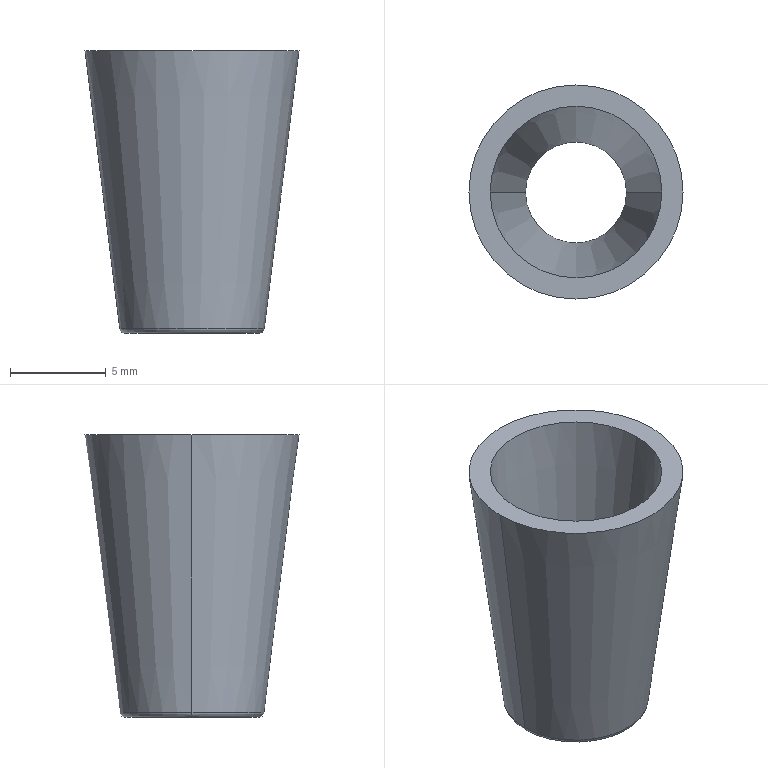Part | SolidWorks | features BaseBody 1 | 1 solid | 8 faces | box 11.2 x 11.2 x 14.8 mm | volume 424.456 mm3 | cone 4 | plane 2 | torus 2
STEP:
#1=CARTESIAN_POINT('',(-298.418,-272.746,351.634));
#2=VERTEX_POINT('',#1);
#3=CARTESIAN_POINT('',(-293.135,-272.746,351.634));
#4=VERTEX_POINT('',#3);
#5=CARTESIAN_POINT('',(-295.776,-272.746,351.634));
#6=DIRECTION('',(0.,0.,-1.));
#7=DIRECTION('',(-1.,0.,0.));
#8=AXIS2_PLACEMENT_3D('',#5,#6,#7);
#9=CIRCLE('',#8,2.641);
#10=EDGE_CURVE('',#2,#4,#9,.T.);
#11=ORIENTED_EDGE('',*,*,#10,.F.);
#12=CARTESIAN_POINT('',(-295.776,-272.746,351.634));
#13=DIRECTION('',(0.,0.,-1.));
#14=DIRECTION('',(1.,0.,0.));
#15=AXIS2_PLACEMENT_3D('',#12,#13,#14);
#16=CIRCLE('',#15,2.641);
#17=EDGE_CURVE('',#4,#2,#16,.T.);
#18=ORIENTED_EDGE('',*,*,#17,.F.);
#19=EDGE_LOOP('',(#11,#18));
#20=FACE_BOUND('',#19,.T.);
#21=CARTESIAN_POINT('',(-299.262,-272.746,351.634));
#22=VERTEX_POINT('',#21);
#23=CARTESIAN_POINT('',(-292.291,-272.746,351.634));
#24=VERTEX_POINT('',#23);
#25=CARTESIAN_POINT('',(-295.776,-272.746,351.634));
#26=DIRECTION('',(0.,0.,1.));
#27=DIRECTION('',(0.9995,-0.03162,0.));
#28=AXIS2_PLACEMENT_3D('',#25,#26,#27);
#29=CIRCLE('',#28,3.485);
#30=EDGE_CURVE('',#22,#24,#29,.T.);
#31=ORIENTED_EDGE('',*,*,#30,.F.);
#32=CARTESIAN_POINT('',(-295.776,-272.746,351.634));
#33=DIRECTION('',(0.,0.,1.));
#34=DIRECTION('',(-0.9995,0.03162,0.));
#35=AXIS2_PLACEMENT_3D('',#32,#33,#34);
#36=CIRCLE('',#35,3.485);
#37=EDGE_CURVE('',#24,#22,#36,.T.);
#38=ORIENTED_EDGE('',*,*,#37,.F.);
#39=EDGE_LOOP('',(#31,#38));
#40=FACE_OUTER_BOUND('',#39,.T.);
#41=CARTESIAN_POINT('',(-295.776,-272.746,351.634));
#42=DIRECTION('',(0.,0.,-1.));
#43=DIRECTION('',(0.,-1.,0.));
#44=AXIS2_PLACEMENT_3D('',#41,#42,#43);
#45=PLANE('',#44);
#46=ADVANCED_FACE('',(#20,#40),#45,.T.);
#47=CARTESIAN_POINT('',(-291.994,-272.746,351.896));
#48=VERTEX_POINT('',#47);
#49=CARTESIAN_POINT('',(-292.291,-272.746,351.934));
#50=DIRECTION('',(0.000000005,1.,0.));
#51=DIRECTION('',(0.9923,-0.000000005,-0.124));
#52=AXIS2_PLACEMENT_3D('',#49,#50,#51);
#53=CIRCLE('',#52,0.3);
#54=EDGE_CURVE('',#48,#24,#53,.T.);
#55=ORIENTED_EDGE('',*,*,#54,.T.);
#56=ORIENTED_EDGE('',*,*,#37,.T.);
#57=CARTESIAN_POINT('',(-299.559,-272.746,351.896));
#58=VERTEX_POINT('',#57);
#59=CARTESIAN_POINT('',(-299.262,-272.746,351.934));
#60=DIRECTION('',(-0.000000005,-1.,0.));
#61=DIRECTION('',(-0.9923,0.000000005,-0.124));
#62=AXIS2_PLACEMENT_3D('',#59,#60,#61);
#63=CIRCLE('',#62,0.3);
#64=EDGE_CURVE('',#58,#22,#63,.T.);
#65=ORIENTED_EDGE('',*,*,#64,.F.);
#66=CARTESIAN_POINT('',(-295.776,-272.746,351.896));
#67=DIRECTION('',(0.,0.,1.));
#68=DIRECTION('',(-0.9995,0.03162,0.));
#69=AXIS2_PLACEMENT_3D('',#66,#67,#68);
#70=CIRCLE('',#69,3.783);
#71=EDGE_CURVE('',#48,#58,#70,.T.);
#72=ORIENTED_EDGE('',*,*,#71,.F.);
#73=EDGE_LOOP('',(#55,#56,#65,#72));
#74=FACE_OUTER_BOUND('',#73,.T.);
#75=CARTESIAN_POINT('',(-295.776,-272.746,351.934));
#76=DIRECTION('',(0.,0.,-1.));
#77=DIRECTION('',(0.9995,-0.03162,0.));
#78=AXIS2_PLACEMENT_3D('',#75,#76,#77);
#79=TOROIDAL_SURFACE('',#78,3.485,0.3);
#80=ADVANCED_FACE('',(#74),#79,.T.);
#81=CARTESIAN_POINT('',(-301.376,-272.746,366.434));
#82=VERTEX_POINT('',#81);
#83=CARTESIAN_POINT('',(-299.559,-272.746,351.896));
#84=DIRECTION('',(-0.124,-0.000000001,0.9923));
#85=VECTOR('',#84,1000.);
#86=LINE('',#83,#85);
#87=EDGE_CURVE('',#58,#82,#86,.T.);
#88=ORIENTED_EDGE('',*,*,#87,.T.);
#89=CARTESIAN_POINT('',(-290.176,-272.746,366.434));
#90=VERTEX_POINT('',#89);
#91=CARTESIAN_POINT('',(-295.776,-272.746,366.434));
#92=DIRECTION('',(0.,0.,-1.));
#93=DIRECTION('',(-1.,0.,0.));
#94=AXIS2_PLACEMENT_3D('',#91,#92,#93);
#95=CIRCLE('',#94,5.6);
#96=EDGE_CURVE('',#82,#90,#95,.T.);
#97=ORIENTED_EDGE('',*,*,#96,.T.);
#98=CARTESIAN_POINT('',(-291.994,-272.746,351.896));
#99=DIRECTION('',(0.124,0.000000001,0.9923));
#100=VECTOR('',#99,1000.);
#101=LINE('',#98,#100);
#102=EDGE_CURVE('',#48,#90,#101,.T.);
#103=ORIENTED_EDGE('',*,*,#102,.F.);
#104=ORIENTED_EDGE('',*,*,#71,.T.);
#105=EDGE_LOOP('',(#88,#97,#103,#104));
#106=FACE_OUTER_BOUND('',#105,.T.);
#107=CARTESIAN_POINT('',(-295.776,-272.746,359.165));
#108=DIRECTION('',(0.,0.,1.));
#109=DIRECTION('',(1.,0.,0.));
#110=AXIS2_PLACEMENT_3D('',#107,#108,#109);
#111=CONICAL_SURFACE('',#110,4.691,0.1244);
#112=ADVANCED_FACE('',(#106),#111,.T.);
#113=ORIENTED_EDGE('',*,*,#102,.T.);
#114=CARTESIAN_POINT('',(-295.776,-272.746,366.434));
#115=DIRECTION('',(0.,0.,-1.));
#116=DIRECTION('',(1.,0.,0.));
#117=AXIS2_PLACEMENT_3D('',#114,#115,#116);
#118=CIRCLE('',#117,5.6);
#119=EDGE_CURVE('',#90,#82,#118,.T.);
#120=ORIENTED_EDGE('',*,*,#119,.T.);
#121=ORIENTED_EDGE('',*,*,#87,.F.);
#122=CARTESIAN_POINT('',(-295.776,-272.746,351.896));
#123=DIRECTION('',(0.,0.,1.));
#124=DIRECTION('',(-1.,0.000000001,0.));
#125=AXIS2_PLACEMENT_3D('',#122,#123,#124);
#126=CIRCLE('',#125,3.783);
#127=EDGE_CURVE('',#58,#48,#126,.T.);
#128=ORIENTED_EDGE('',*,*,#127,.T.);
#129=EDGE_LOOP('',(#113,#120,#121,#128));
#130=FACE_OUTER_BOUND('',#129,.T.);
#131=CARTESIAN_POINT('',(-295.776,-272.746,359.165));
#132=DIRECTION('',(0.,0.,1.));
#133=DIRECTION('',(1.,0.,0.));
#134=AXIS2_PLACEMENT_3D('',#131,#132,#133);
#135=CONICAL_SURFACE('',#134,4.691,0.1244);
#136=ADVANCED_FACE('',(#130),#135,.T.);
#137=ORIENTED_EDGE('',*,*,#64,.T.);
#138=ORIENTED_EDGE('',*,*,#30,.T.);
#139=ORIENTED_EDGE('',*,*,#54,.F.);
#140=ORIENTED_EDGE('',*,*,#127,.F.);
#141=EDGE_LOOP('',(#137,#138,#139,#140));
#142=FACE_OUTER_BOUND('',#141,.T.);
#143=CARTESIAN_POINT('',(-295.776,-272.746,351.934));
#144=DIRECTION('',(0.,0.,-1.));
#145=DIRECTION('',(-0.9995,0.03162,0.));
#146=AXIS2_PLACEMENT_3D('',#143,#144,#145);
#147=TOROIDAL_SURFACE('',#146,3.485,0.3);
#148=ADVANCED_FACE('',(#142),#147,.T.);
#149=CARTESIAN_POINT('',(-291.285,-272.746,366.434));
#150=VERTEX_POINT('',#149);
#151=CARTESIAN_POINT('',(-300.268,-272.746,366.434));
#152=VERTEX_POINT('',#151);
#153=CARTESIAN_POINT('',(-295.776,-272.746,366.434));
#154=DIRECTION('',(0.,0.,1.));
#155=DIRECTION('',(1.,0.,0.));
#156=AXIS2_PLACEMENT_3D('',#153,#154,#155);
#157=CIRCLE('',#156,4.491);
#158=EDGE_CURVE('',#150,#152,#157,.T.);
#159=ORIENTED_EDGE('',*,*,#158,.F.);
#160=CARTESIAN_POINT('',(-295.776,-272.746,366.434));
#161=DIRECTION('',(0.,0.,1.));
#162=DIRECTION('',(-1.,0.,0.));
#163=AXIS2_PLACEMENT_3D('',#160,#161,#162);
#164=CIRCLE('',#163,4.491);
#165=EDGE_CURVE('',#152,#150,#164,.T.);
#166=ORIENTED_EDGE('',*,*,#165,.F.);
#167=EDGE_LOOP('',(#159,#166));
#168=FACE_BOUND('',#167,.T.);
#169=ORIENTED_EDGE('',*,*,#119,.F.);
#170=ORIENTED_EDGE('',*,*,#96,.F.);
#171=EDGE_LOOP('',(#169,#170));
#172=FACE_OUTER_BOUND('',#171,.T.);
#173=CARTESIAN_POINT('',(-295.776,-272.746,366.434));
#174=DIRECTION('',(0.,0.,-1.));
#175=DIRECTION('',(0.,-1.,0.));
#176=AXIS2_PLACEMENT_3D('',#173,#174,#175);
#177=PLANE('',#176);
#178=ADVANCED_FACE('',(#168,#172),#177,.F.);
#179=CARTESIAN_POINT('',(-298.418,-272.746,351.634));
#180=DIRECTION('',(-0.124,0.,0.9923));
#181=VECTOR('',#180,1000.);
#182=LINE('',#179,#181);
#183=EDGE_CURVE('',#2,#152,#182,.T.);
#184=ORIENTED_EDGE('',*,*,#183,.T.);
#185=ORIENTED_EDGE('',*,*,#165,.T.);
#186=CARTESIAN_POINT('',(-293.135,-272.746,351.634));
#187=DIRECTION('',(0.124,0.,0.9923));
#188=VECTOR('',#187,1000.);
#189=LINE('',#186,#188);
#190=EDGE_CURVE('',#4,#150,#189,.T.);
#191=ORIENTED_EDGE('',*,*,#190,.F.);
#192=ORIENTED_EDGE('',*,*,#17,.T.);
#193=EDGE_LOOP('',(#184,#185,#191,#192));
#194=FACE_OUTER_BOUND('',#193,.T.);
#195=CARTESIAN_POINT('',(-295.776,-272.746,359.034));
#196=DIRECTION('',(0.,0.,1.));
#197=DIRECTION('',(1.,0.,0.));
#198=AXIS2_PLACEMENT_3D('',#195,#196,#197);
#199=CONICAL_SURFACE('',#198,3.566,0.1244);
#200=ADVANCED_FACE('',(#194),#199,.F.);
#201=ORIENTED_EDGE('',*,*,#190,.T.);
#202=ORIENTED_EDGE('',*,*,#158,.T.);
#203=ORIENTED_EDGE('',*,*,#183,.F.);
#204=ORIENTED_EDGE('',*,*,#10,.T.);
#205=EDGE_LOOP('',(#201,#202,#203,#204));
#206=FACE_OUTER_BOUND('',#205,.T.);
#207=CARTESIAN_POINT('',(-295.776,-272.746,359.034));
#208=DIRECTION('',(0.,0.,1.));
#209=DIRECTION('',(1.,0.,0.));
#210=AXIS2_PLACEMENT_3D('',#207,#208,#209);
#211=CONICAL_SURFACE('',#210,3.566,0.1244);
#212=ADVANCED_FACE('',(#206),#211,.F.);
#213=CLOSED_SHELL('',(#46,#80,#112,#136,#148,#178,#200,#212));
#214=MANIFOLD_SOLID_BREP('',#213);
#215=CARTESIAN_POINT('',(0.,0.,0.));
#216=DIRECTION('',(0.,0.,1.));
#217=DIRECTION('',(1.,0.,0.));
#218=AXIS2_PLACEMENT_3D('',#215,#216,#217);
#219=(LENGTH_UNIT()NAMED_UNIT(*)SI_UNIT(.MILLI.,.METRE.));
#220=UNCERTAINTY_MEASURE_WITH_UNIT(LENGTH_MEASURE(0.00001),#219,'','');
#221=(NAMED_UNIT(*)PLANE_ANGLE_UNIT()SI_UNIT($,.RADIAN.));
#222=(NAMED_UNIT(*)SI_UNIT($,.STERADIAN.)SOLID_ANGLE_UNIT());
#223=(GEOMETRIC_REPRESENTATION_CONTEXT(3)GLOBAL_UNCERTAINTY_ASSIGNED_CONTEXT((#220))GLOBAL_UNIT_ASSIGNED_CONTEXT((#219,#221,#222))REPRESENTATION_CONTEXT('',''));
#224=ADVANCED_BREP_SHAPE_REPRESENTATION('',(#214,#218),#223);